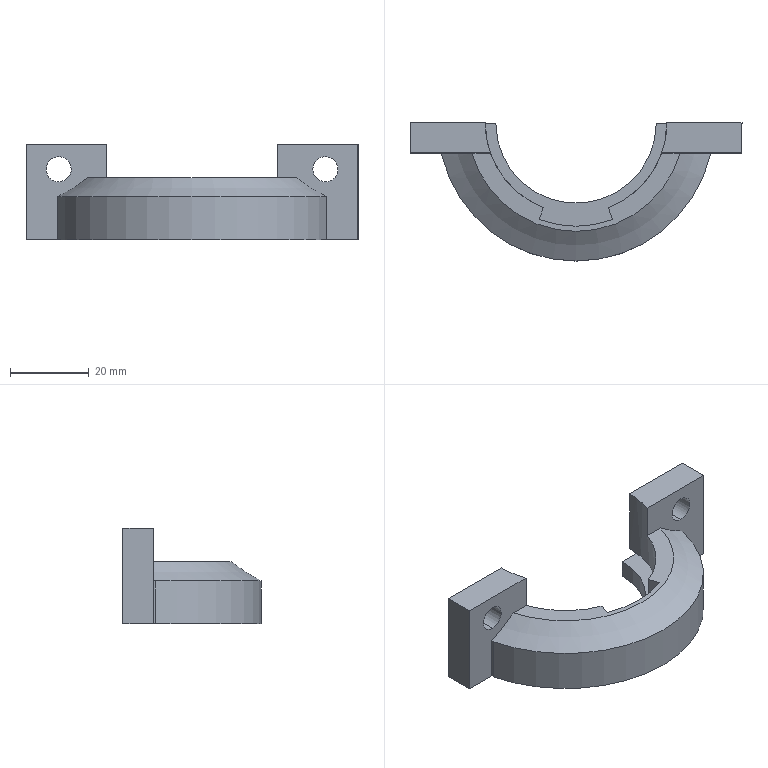Part | SolidWorks | features ICE 14, 3DProfileFeature 1, Cut 1, Extrusion 1, Fillet 1, HoleWzd 1, MirrorPattern 1, MirrorSolid 1, RefAxis 1, RevCut 1, Revolution 1, SewRefSurface 1, Sweep 1, Thicken 1 | 1 solid | 29 faces | box 84.091 x 34.963 x 24.206 mm | volume 18007 mm3 | plane 18 | cylinder 6 | spline 4 | torus 1 | commonest cylinder face diameters 45.974 x2 40.64 x1 52.324 x1 59.436 x1 69.927 x1
STEP:
#1=CARTESIAN_POINT('',(33.782,0.,13.792));
#2=VERTEX_POINT('',#1);
#3=CARTESIAN_POINT('',(33.782,0.,7.442));
#4=VERTEX_POINT('',#3);
#5=CARTESIAN_POINT('',(33.782,0.,13.792));
#6=CARTESIAN_POINT('',(40.132,0.,13.792));
#7=CARTESIAN_POINT('',(40.132,0.,7.442));
#8=CARTESIAN_POINT('',(33.782,0.,7.442));
#9=(BOUNDED_CURVE()B_SPLINE_CURVE(3,(#5,#6,#7,#8),.UNSPECIFIED.,.F.,.F.)B_SPLINE_CURVE_WITH_KNOTS((4,4),(0.,3.142),.UNSPECIFIED.)CURVE()GEOMETRIC_REPRESENTATION_ITEM()RATIONAL_B_SPLINE_CURVE((1.,0.3333,0.3333,1.))REPRESENTATION_ITEM(''));
#10=EDGE_CURVE('',#2,#4,#9,.T.);
#11=ORIENTED_EDGE('',*,*,#10,.T.);
#12=CARTESIAN_POINT('',(33.782,-7.62,7.442));
#13=VERTEX_POINT('',#12);
#14=CARTESIAN_POINT('',(33.782,10.16,7.442));
#15=DIRECTION('',(0.,-1.,0.));
#16=VECTOR('',#15,1000.);
#17=LINE('',#14,#16);
#18=EDGE_CURVE('',#4,#13,#17,.T.);
#19=ORIENTED_EDGE('',*,*,#18,.T.);
#20=CARTESIAN_POINT('',(33.782,-7.62,13.792));
#21=VERTEX_POINT('',#20);
#22=CARTESIAN_POINT('',(33.782,-7.62,13.792));
#23=CARTESIAN_POINT('',(40.132,-7.62,13.792));
#24=CARTESIAN_POINT('',(40.132,-7.62,7.442));
#25=CARTESIAN_POINT('',(33.782,-7.62,7.442));
#26=(BOUNDED_CURVE()B_SPLINE_CURVE(3,(#22,#23,#24,#25),.UNSPECIFIED.,.F.,.F.)B_SPLINE_CURVE_WITH_KNOTS((4,4),(0.,3.142),.UNSPECIFIED.)CURVE()GEOMETRIC_REPRESENTATION_ITEM()RATIONAL_B_SPLINE_CURVE((1.,0.3333,0.3333,1.))REPRESENTATION_ITEM(''));
#27=EDGE_CURVE('',#21,#13,#26,.T.);
#28=ORIENTED_EDGE('',*,*,#27,.F.);
#29=CARTESIAN_POINT('',(33.782,10.16,13.792));
#30=DIRECTION('',(0.,-1.,0.));
#31=VECTOR('',#30,1000.);
#32=LINE('',#29,#31);
#33=EDGE_CURVE('',#2,#21,#32,.T.);
#34=ORIENTED_EDGE('',*,*,#33,.F.);
#35=EDGE_LOOP('',(#11,#19,#28,#34));
#36=FACE_OUTER_BOUND('',#35,.T.);
#37=CARTESIAN_POINT('',(33.782,0.,13.792));
#38=CARTESIAN_POINT('',(33.782,-7.62,13.792));
#39=CARTESIAN_POINT('',(40.132,0.,13.792));
#40=CARTESIAN_POINT('',(40.132,-7.62,13.792));
#41=CARTESIAN_POINT('',(40.132,0.,7.442));
#42=CARTESIAN_POINT('',(40.132,-7.62,7.442));
#43=CARTESIAN_POINT('',(33.782,0.,7.442));
#44=CARTESIAN_POINT('',(33.782,-7.62,7.442));
#45=(BOUNDED_SURFACE()B_SPLINE_SURFACE(3,1,((#37,#38),(#39,#40),(#41,#42),(#43,#44)),.UNSPECIFIED.,.F.,.F.,.T.)B_SPLINE_SURFACE_WITH_KNOTS((4,4),(2,2),(0.,1.),(0.,1.),.UNSPECIFIED.)GEOMETRIC_REPRESENTATION_ITEM()RATIONAL_B_SPLINE_SURFACE(((1.,1.),(0.3333,0.3333),(0.3333,0.3333),(1.,1.)))REPRESENTATION_ITEM('')SURFACE());
#46=ADVANCED_FACE('',(#36),#45,.T.);
#47=CARTESIAN_POINT('',(-33.782,0.,7.442));
#48=VERTEX_POINT('',#47);
#49=CARTESIAN_POINT('',(-33.782,0.,13.792));
#50=VERTEX_POINT('',#49);
#51=CARTESIAN_POINT('',(-33.782,0.,7.442));
#52=CARTESIAN_POINT('',(-27.432,0.,7.442));
#53=CARTESIAN_POINT('',(-27.432,0.,13.792));
#54=CARTESIAN_POINT('',(-33.782,0.,13.792));
#55=(BOUNDED_CURVE()B_SPLINE_CURVE(3,(#51,#52,#53,#54),.UNSPECIFIED.,.F.,.T.)B_SPLINE_CURVE_WITH_KNOTS((4,4),(3.142,6.283),.UNSPECIFIED.)CURVE()GEOMETRIC_REPRESENTATION_ITEM()RATIONAL_B_SPLINE_CURVE((1.,0.3333,0.3333,1.))REPRESENTATION_ITEM(''));
#56=EDGE_CURVE('',#48,#50,#55,.T.);
#57=ORIENTED_EDGE('',*,*,#56,.F.);
#58=CARTESIAN_POINT('',(-33.782,-7.62,7.442));
#59=VERTEX_POINT('',#58);
#60=CARTESIAN_POINT('',(-33.782,10.16,7.442));
#61=DIRECTION('',(0.,-1.,0.));
#62=VECTOR('',#61,1000.);
#63=LINE('',#60,#62);
#64=EDGE_CURVE('',#48,#59,#63,.T.);
#65=ORIENTED_EDGE('',*,*,#64,.T.);
#66=CARTESIAN_POINT('',(-33.782,-7.62,13.792));
#67=VERTEX_POINT('',#66);
#68=CARTESIAN_POINT('',(-33.782,-7.62,7.442));
#69=CARTESIAN_POINT('',(-27.432,-7.62,7.442));
#70=CARTESIAN_POINT('',(-27.432,-7.62,13.792));
#71=CARTESIAN_POINT('',(-33.782,-7.62,13.792));
#72=(BOUNDED_CURVE()B_SPLINE_CURVE(3,(#68,#69,#70,#71),.UNSPECIFIED.,.F.,.T.)B_SPLINE_CURVE_WITH_KNOTS((4,4),(3.142,6.283),.UNSPECIFIED.)CURVE()GEOMETRIC_REPRESENTATION_ITEM()RATIONAL_B_SPLINE_CURVE((1.,0.3333,0.3333,1.))REPRESENTATION_ITEM(''));
#73=EDGE_CURVE('',#59,#67,#72,.T.);
#74=ORIENTED_EDGE('',*,*,#73,.T.);
#75=CARTESIAN_POINT('',(-33.782,10.16,13.792));
#76=DIRECTION('',(0.,-1.,0.));
#77=VECTOR('',#76,1000.);
#78=LINE('',#75,#77);
#79=EDGE_CURVE('',#50,#67,#78,.T.);
#80=ORIENTED_EDGE('',*,*,#79,.F.);
#81=EDGE_LOOP('',(#57,#65,#74,#80));
#82=FACE_OUTER_BOUND('',#81,.T.);
#83=CARTESIAN_POINT('',(-33.782,0.,7.442));
#84=CARTESIAN_POINT('',(-33.782,-7.62,7.442));
#85=CARTESIAN_POINT('',(-27.432,0.,7.442));
#86=CARTESIAN_POINT('',(-27.432,-7.62,7.442));
#87=CARTESIAN_POINT('',(-27.432,0.,13.792));
#88=CARTESIAN_POINT('',(-27.432,-7.62,13.792));
#89=CARTESIAN_POINT('',(-33.782,0.,13.792));
#90=CARTESIAN_POINT('',(-33.782,-7.62,13.792));
#91=(BOUNDED_SURFACE()B_SPLINE_SURFACE(3,1,((#83,#84),(#85,#86),(#87,#88),(#89,#90)),.UNSPECIFIED.,.F.,.F.,.F.)B_SPLINE_SURFACE_WITH_KNOTS((4,4),(2,2),(0.,1.),(0.,1.),.UNSPECIFIED.)GEOMETRIC_REPRESENTATION_ITEM()RATIONAL_B_SPLINE_SURFACE(((1.,1.),(0.3333,0.3333),(0.3333,0.3333),(1.,1.)))REPRESENTATION_ITEM('')SURFACE());
#92=ADVANCED_FACE('',(#82),#91,.F.);
#93=CARTESIAN_POINT('',(20.32,0.,-2.778));
#94=VERTEX_POINT('',#93);
#95=CARTESIAN_POINT('',(-20.32,0.,-2.778));
#96=VERTEX_POINT('',#95);
#97=CARTESIAN_POINT('',(0.,0.,-2.778));
#98=DIRECTION('',(0.,0.,-1.));
#99=DIRECTION('',(1.,0.,0.));
#100=AXIS2_PLACEMENT_3D('',#97,#98,#99);
#101=CIRCLE('',#100,20.32);
#102=EDGE_CURVE('',#94,#96,#101,.T.);
#103=ORIENTED_EDGE('',*,*,#102,.F.);
#104=CARTESIAN_POINT('',(20.32,0.,-7.239));
#105=VERTEX_POINT('',#104);
#106=CARTESIAN_POINT('',(20.32,0.,87.108));
#107=DIRECTION('',(0.,0.,-1.));
#108=VECTOR('',#107,1000.);
#109=LINE('',#106,#108);
#110=EDGE_CURVE('',#94,#105,#109,.T.);
#111=ORIENTED_EDGE('',*,*,#110,.T.);
#112=CARTESIAN_POINT('',(-20.32,0.,-7.239));
#113=VERTEX_POINT('',#112);
#114=CARTESIAN_POINT('',(0.,0.,-7.239));
#115=DIRECTION('',(0.,0.,-1.));
#116=DIRECTION('',(-1.,0.,0.));
#117=AXIS2_PLACEMENT_3D('',#114,#115,#116);
#118=CIRCLE('',#117,20.32);
#119=EDGE_CURVE('',#105,#113,#118,.T.);
#120=ORIENTED_EDGE('',*,*,#119,.T.);
#121=CARTESIAN_POINT('',(-20.32,0.,87.108));
#122=DIRECTION('',(0.,0.,1.));
#123=VECTOR('',#122,1000.);
#124=LINE('',#121,#123);
#125=EDGE_CURVE('',#113,#96,#124,.T.);
#126=ORIENTED_EDGE('',*,*,#125,.T.);
#127=EDGE_LOOP('',(#103,#111,#120,#126));
#128=FACE_OUTER_BOUND('',#127,.T.);
#129=CARTESIAN_POINT('',(0.,0.,87.108));
#130=DIRECTION('',(0.,0.,-1.));
#131=DIRECTION('',(-1.,0.,0.));
#132=AXIS2_PLACEMENT_3D('',#129,#130,#131);
#133=CYLINDRICAL_SURFACE('',#132,20.32);
#134=ADVANCED_FACE('',(#128),#133,.F.);
#135=ORIENTED_EDGE('',*,*,#27,.T.);
#136=CARTESIAN_POINT('',(33.782,-7.62,7.442));
#137=CARTESIAN_POINT('',(27.432,-7.62,7.442));
#138=CARTESIAN_POINT('',(27.432,-7.62,13.792));
#139=CARTESIAN_POINT('',(33.782,-7.62,13.792));
#140=(BOUNDED_CURVE()B_SPLINE_CURVE(3,(#136,#137,#138,#139),.UNSPECIFIED.,.F.,.F.)B_SPLINE_CURVE_WITH_KNOTS((4,4),(3.142,6.283),.UNSPECIFIED.)CURVE()GEOMETRIC_REPRESENTATION_ITEM()RATIONAL_B_SPLINE_CURVE((1.,0.3333,0.3333,1.))REPRESENTATION_ITEM(''));
#141=EDGE_CURVE('',#13,#21,#140,.T.);
#142=ORIENTED_EDGE('',*,*,#141,.T.);
#143=EDGE_LOOP('',(#135,#142));
#144=FACE_BOUND('',#143,.T.);
#145=CARTESIAN_POINT('',(21.687,-7.62,8.484));
#146=VERTEX_POINT('',#145);
#147=CARTESIAN_POINT('',(26.377,-7.62,8.484));
#148=VERTEX_POINT('',#147);
#149=CARTESIAN_POINT('',(0.,-7.62,8.484));
#150=DIRECTION('',(1.,0.,0.));
#151=VECTOR('',#150,1000.);
#152=LINE('',#149,#151);
#153=EDGE_CURVE('',#146,#148,#152,.T.);
#154=ORIENTED_EDGE('',*,*,#153,.T.);
#155=CARTESIAN_POINT('',(33.984,-7.62,3.706));
#156=VERTEX_POINT('',#155);
#157=CARTESIAN_POINT('',(26.377,-7.62,8.484));
#158=CARTESIAN_POINT('',(28.729,-7.62,6.598));
#159=CARTESIAN_POINT('',(31.263,-7.62,5.003));
#160=CARTESIAN_POINT('',(33.984,-7.62,3.706));
#161=B_SPLINE_CURVE_WITH_KNOTS('',3,(#157,#158,#159,#160),.UNSPECIFIED.,.F.,.F.,(4,4),(0.,0.008983),.UNSPECIFIED.);
#162=EDGE_CURVE('',#148,#156,#161,.T.);
#163=ORIENTED_EDGE('',*,*,#162,.T.);
#164=CARTESIAN_POINT('',(33.984,-7.62,-7.239));
#165=VERTEX_POINT('',#164);
#166=CARTESIAN_POINT('',(33.984,-7.62,2.54));
#167=DIRECTION('',(0.,0.,-1.));
#168=VECTOR('',#167,1000.);
#169=LINE('',#166,#168);
#170=EDGE_CURVE('',#156,#165,#169,.T.);
#171=ORIENTED_EDGE('',*,*,#170,.T.);
#172=CARTESIAN_POINT('',(42.02,-7.62,-7.239));
#173=VERTEX_POINT('',#172);
#174=CARTESIAN_POINT('',(0.,-7.62,-7.239));
#175=DIRECTION('',(-1.,0.,0.));
#176=VECTOR('',#175,1000.);
#177=LINE('',#174,#176);
#178=EDGE_CURVE('',#173,#165,#177,.T.);
#179=ORIENTED_EDGE('',*,*,#178,.F.);
#180=CARTESIAN_POINT('',(42.02,-7.62,16.967));
#181=VERTEX_POINT('',#180);
#182=CARTESIAN_POINT('',(42.02,-7.62,16.967));
#183=DIRECTION('',(0.,0.,-1.));
#184=VECTOR('',#183,1000.);
#185=LINE('',#182,#184);
#186=EDGE_CURVE('',#181,#173,#185,.T.);
#187=ORIENTED_EDGE('',*,*,#186,.F.);
#188=CARTESIAN_POINT('',(21.687,-7.62,16.967));
#189=VERTEX_POINT('',#188);
#190=CARTESIAN_POINT('',(0.,-7.62,16.967));
#191=DIRECTION('',(-1.,0.,0.));
#192=VECTOR('',#191,1000.);
#193=LINE('',#190,#192);
#194=EDGE_CURVE('',#181,#189,#193,.T.);
#195=ORIENTED_EDGE('',*,*,#194,.T.);
#196=CARTESIAN_POINT('',(21.687,-7.62,8.484));
#197=DIRECTION('',(0.,0.,1.));
#198=VECTOR('',#197,1000.);
#199=LINE('',#196,#198);
#200=EDGE_CURVE('',#146,#189,#199,.T.);
#201=ORIENTED_EDGE('',*,*,#200,.F.);
#202=EDGE_LOOP('',(#154,#163,#171,#179,#187,#195,#201));
#203=FACE_OUTER_BOUND('',#202,.T.);
#204=CARTESIAN_POINT('',(0.,-7.62,0.));
#205=DIRECTION('',(0.,-1.,0.));
#206=DIRECTION('',(0.,0.,-1.));
#207=AXIS2_PLACEMENT_3D('',#204,#205,#206);
#208=PLANE('',#207);
#209=ADVANCED_FACE('',(#144,#203),#208,.T.);
#210=CARTESIAN_POINT('',(9.312,-24.448,8.484));
#211=VERTEX_POINT('',#210);
#212=CARTESIAN_POINT('',(9.312,-24.448,0.));
#213=VERTEX_POINT('',#212);
#214=CARTESIAN_POINT('',(9.312,-24.448,7.137));
#215=DIRECTION('',(0.,0.,-1.));
#216=VECTOR('',#215,1000.);
#217=LINE('',#214,#216);
#218=EDGE_CURVE('',#211,#213,#217,.T.);
#219=ORIENTED_EDGE('',*,*,#218,.F.);
#220=CARTESIAN_POINT('',(8.182,-21.481,8.484));
#221=VERTEX_POINT('',#220);
#222=CARTESIAN_POINT('',(0.,0.,8.484));
#223=DIRECTION('',(0.356,-0.9345,0.));
#224=VECTOR('',#223,1000.);
#225=LINE('',#222,#224);
#226=EDGE_CURVE('',#221,#211,#225,.T.);
#227=ORIENTED_EDGE('',*,*,#226,.F.);
#228=CARTESIAN_POINT('',(8.182,-21.481,0.));
#229=VERTEX_POINT('',#228);
#230=CARTESIAN_POINT('',(8.182,-21.481,16.967));
#231=DIRECTION('',(0.,0.,1.));
#232=VECTOR('',#231,1000.);
#233=LINE('',#230,#232);
#234=EDGE_CURVE('',#229,#221,#233,.T.);
#235=ORIENTED_EDGE('',*,*,#234,.F.);
#236=CARTESIAN_POINT('',(0.,0.,0.));
#237=DIRECTION('',(0.356,-0.9345,0.));
#238=VECTOR('',#237,1000.);
#239=LINE('',#236,#238);
#240=EDGE_CURVE('',#229,#213,#239,.T.);
#241=ORIENTED_EDGE('',*,*,#240,.T.);
#242=EDGE_LOOP('',(#219,#227,#235,#241));
#243=FACE_OUTER_BOUND('',#242,.T.);
#244=CARTESIAN_POINT('',(0.,0.,-0.8128));
#245=DIRECTION('',(-0.9345,-0.356,0.));
#246=DIRECTION('',(0.356,-0.9345,0.));
#247=AXIS2_PLACEMENT_3D('',#244,#245,#246);
#248=PLANE('',#247);
#249=ADVANCED_FACE('',(#243),#248,.T.);
#250=CARTESIAN_POINT('',(22.987,0.,16.967));
#251=VERTEX_POINT('',#250);
#252=CARTESIAN_POINT('',(0.,0.,16.967));
#253=DIRECTION('',(0.,0.,1.));
#254=DIRECTION('',(1.,0.,0.));
#255=AXIS2_PLACEMENT_3D('',#252,#253,#254);
#256=CIRCLE('',#255,22.987);
#257=EDGE_CURVE('',#189,#251,#256,.T.);
#258=ORIENTED_EDGE('',*,*,#257,.F.);
#259=ORIENTED_EDGE('',*,*,#194,.F.);
#260=CARTESIAN_POINT('',(42.037,0.,16.967));
#261=VERTEX_POINT('',#260);
#262=CARTESIAN_POINT('',(42.037,0.05675,16.967));
#263=DIRECTION('',(-0.002237,-1.,0.));
#264=VECTOR('',#263,1000.);
#265=LINE('',#262,#264);
#266=EDGE_CURVE('',#261,#181,#265,.T.);
#267=ORIENTED_EDGE('',*,*,#266,.F.);
#268=CARTESIAN_POINT('',(0.,0.,16.967));
#269=DIRECTION('',(1.,0.,0.));
#270=VECTOR('',#269,1000.);
#271=LINE('',#268,#270);
#272=EDGE_CURVE('',#251,#261,#271,.T.);
#273=ORIENTED_EDGE('',*,*,#272,.F.);
#274=EDGE_LOOP('',(#258,#259,#267,#273));
#275=FACE_OUTER_BOUND('',#274,.T.);
#276=CARTESIAN_POINT('',(0.,0.,16.967));
#277=DIRECTION('',(0.,0.,1.));
#278=DIRECTION('',(1.,0.,0.));
#279=AXIS2_PLACEMENT_3D('',#276,#277,#278);
#280=PLANE('',#279);
#281=ADVANCED_FACE('',(#275),#280,.T.);
#282=CARTESIAN_POINT('',(0.,0.,8.484));
#283=DIRECTION('',(0.,0.,-1.));
#284=DIRECTION('',(1.,0.,0.));
#285=AXIS2_PLACEMENT_3D('',#282,#283,#284);
#286=CIRCLE('',#285,22.987);
#287=EDGE_CURVE('',#146,#221,#286,.T.);
#288=ORIENTED_EDGE('',*,*,#287,.F.);
#289=ORIENTED_EDGE('',*,*,#200,.T.);
#290=ORIENTED_EDGE('',*,*,#257,.T.);
#291=CARTESIAN_POINT('',(22.987,0.,0.));
#292=VERTEX_POINT('',#291);
#293=CARTESIAN_POINT('',(22.987,0.,16.967));
#294=DIRECTION('',(0.,0.,1.));
#295=VECTOR('',#294,1000.);
#296=LINE('',#293,#295);
#297=EDGE_CURVE('',#292,#251,#296,.T.);
#298=ORIENTED_EDGE('',*,*,#297,.F.);
#299=CARTESIAN_POINT('',(0.,0.,0.));
#300=DIRECTION('',(0.,0.,1.));
#301=DIRECTION('',(1.,0.,0.));
#302=AXIS2_PLACEMENT_3D('',#299,#300,#301);
#303=CIRCLE('',#302,22.987);
#304=EDGE_CURVE('',#229,#292,#303,.T.);
#305=ORIENTED_EDGE('',*,*,#304,.F.);
#306=ORIENTED_EDGE('',*,*,#234,.T.);
#307=EDGE_LOOP('',(#288,#289,#290,#298,#305,#306));
#308=FACE_OUTER_BOUND('',#307,.T.);
#309=CARTESIAN_POINT('',(0.,0.,16.967));
#310=DIRECTION('',(0.,0.,-1.));
#311=DIRECTION('',(-1.,0.,0.));
#312=AXIS2_PLACEMENT_3D('',#309,#310,#311);
#313=CYLINDRICAL_SURFACE('',#312,22.987);
#314=ADVANCED_FACE('',(#308),#313,.F.);
#315=CARTESIAN_POINT('',(-9.312,-24.448,8.484));
#316=VERTEX_POINT('',#315);
#317=CARTESIAN_POINT('',(-8.293,-21.439,8.484));
#318=VERTEX_POINT('',#317);
#319=CARTESIAN_POINT('',(-0.921,0.3121,8.484));
#320=DIRECTION('',(0.321,0.9471,0.));
#321=VECTOR('',#320,1000.);
#322=LINE('',#319,#321);
#323=EDGE_CURVE('',#316,#318,#322,.T.);
#324=ORIENTED_EDGE('',*,*,#323,.F.);
#325=CARTESIAN_POINT('',(-9.312,-24.448,0.));
#326=VERTEX_POINT('',#325);
#327=CARTESIAN_POINT('',(-9.312,-24.448,7.137));
#328=DIRECTION('',(0.,0.,-1.));
#329=VECTOR('',#328,1000.);
#330=LINE('',#327,#329);
#331=EDGE_CURVE('',#316,#326,#330,.T.);
#332=ORIENTED_EDGE('',*,*,#331,.T.);
#333=CARTESIAN_POINT('',(-8.293,-21.439,0.));
#334=VERTEX_POINT('',#333);
#335=CARTESIAN_POINT('',(-0.921,0.3121,0.));
#336=DIRECTION('',(-0.321,-0.9471,0.));
#337=VECTOR('',#336,1000.);
#338=LINE('',#335,#337);
#339=EDGE_CURVE('',#334,#326,#338,.T.);
#340=ORIENTED_EDGE('',*,*,#339,.F.);
#341=CARTESIAN_POINT('',(-8.293,-21.439,16.967));
#342=DIRECTION('',(0.,0.,1.));
#343=VECTOR('',#342,1000.);
#344=LINE('',#341,#343);
#345=EDGE_CURVE('',#334,#318,#344,.T.);
#346=ORIENTED_EDGE('',*,*,#345,.T.);
#347=EDGE_LOOP('',(#324,#332,#340,#346));
#348=FACE_OUTER_BOUND('',#347,.T.);
#349=CARTESIAN_POINT('',(-0.921,0.3121,-0.8128));
#350=DIRECTION('',(-0.9471,0.321,0.));
#351=DIRECTION('',(-0.321,-0.9471,0.));
#352=AXIS2_PLACEMENT_3D('',#349,#350,#351);
#353=PLANE('',#352);
#354=ADVANCED_FACE('',(#348),#353,.F.);
#355=CARTESIAN_POINT('',(-42.054,-7.62,16.967));
#356=VERTEX_POINT('',#355);
#357=CARTESIAN_POINT('',(-21.687,-7.62,16.967));
#358=VERTEX_POINT('',#357);
#359=CARTESIAN_POINT('',(0.,-7.62,16.967));
#360=DIRECTION('',(1.,0.,0.));
#361=VECTOR('',#360,1000.);
#362=LINE('',#359,#361);
#363=EDGE_CURVE('',#356,#358,#362,.T.);
#364=ORIENTED_EDGE('',*,*,#363,.T.);
#365=CARTESIAN_POINT('',(-22.987,0.,16.967));
#366=VERTEX_POINT('',#365);
#367=CARTESIAN_POINT('',(0.,0.,16.967));
#368=DIRECTION('',(0.,0.,1.));
#369=DIRECTION('',(1.,0.,0.));
#370=AXIS2_PLACEMENT_3D('',#367,#368,#369);
#371=CIRCLE('',#370,22.987);
#372=EDGE_CURVE('',#366,#358,#371,.T.);
#373=ORIENTED_EDGE('',*,*,#372,.F.);
#374=CARTESIAN_POINT('',(-42.037,0.,16.967));
#375=VERTEX_POINT('',#374);
#376=CARTESIAN_POINT('',(0.,0.,16.967));
#377=DIRECTION('',(1.,0.,0.));
#378=VECTOR('',#377,1000.);
#379=LINE('',#376,#378);
#380=EDGE_CURVE('',#375,#366,#379,.T.);
#381=ORIENTED_EDGE('',*,*,#380,.F.);
#382=CARTESIAN_POINT('',(-42.054,-7.677,16.967));
#383=DIRECTION('',(-0.002237,-1.,0.));
#384=VECTOR('',#383,1000.);
#385=LINE('',#382,#384);
#386=EDGE_CURVE('',#375,#356,#385,.T.);
#387=ORIENTED_EDGE('',*,*,#386,.T.);
#388=EDGE_LOOP('',(#364,#373,#381,#387));
#389=FACE_OUTER_BOUND('',#388,.T.);
#390=CARTESIAN_POINT('',(0.,0.,16.967));
#391=DIRECTION('',(0.,0.,1.));
#392=DIRECTION('',(1.,0.,0.));
#393=AXIS2_PLACEMENT_3D('',#390,#391,#392);
#394=PLANE('',#393);
#395=ADVANCED_FACE('',(#389),#394,.T.);
#396=ORIENTED_EDGE('',*,*,#372,.T.);
#397=CARTESIAN_POINT('',(-21.687,-7.62,8.484));
#398=VERTEX_POINT('',#397);
#399=CARTESIAN_POINT('',(-21.687,-7.62,8.484));
#400=DIRECTION('',(0.,0.,1.));
#401=VECTOR('',#400,1000.);
#402=LINE('',#399,#401);
#403=EDGE_CURVE('',#398,#358,#402,.T.);
#404=ORIENTED_EDGE('',*,*,#403,.F.);
#405=CARTESIAN_POINT('',(0.,0.,8.484));
#406=DIRECTION('',(0.,0.,1.));
#407=DIRECTION('',(1.,0.,0.));
#408=AXIS2_PLACEMENT_3D('',#405,#406,#407);
#409=CIRCLE('',#408,22.987);
#410=EDGE_CURVE('',#398,#318,#409,.T.);
#411=ORIENTED_EDGE('',*,*,#410,.T.);
#412=ORIENTED_EDGE('',*,*,#345,.F.);
#413=CARTESIAN_POINT('',(-22.987,0.,0.));
#414=VERTEX_POINT('',#413);
#415=CARTESIAN_POINT('',(0.,0.,0.));
#416=DIRECTION('',(0.,0.,1.));
#417=DIRECTION('',(1.,0.,0.));
#418=AXIS2_PLACEMENT_3D('',#415,#416,#417);
#419=CIRCLE('',#418,22.987);
#420=EDGE_CURVE('',#414,#334,#419,.T.);
#421=ORIENTED_EDGE('',*,*,#420,.F.);
#422=CARTESIAN_POINT('',(-22.987,0.,16.967));
#423=DIRECTION('',(0.,0.,-1.));
#424=VECTOR('',#423,1000.);
#425=LINE('',#422,#424);
#426=EDGE_CURVE('',#366,#414,#425,.T.);
#427=ORIENTED_EDGE('',*,*,#426,.F.);
#428=EDGE_LOOP('',(#396,#404,#411,#412,#421,#427));
#429=FACE_OUTER_BOUND('',#428,.T.);
#430=CARTESIAN_POINT('',(0.,0.,16.967));
#431=DIRECTION('',(0.,0.,-1.));
#432=DIRECTION('',(-1.,0.,0.));
#433=AXIS2_PLACEMENT_3D('',#430,#431,#432);
#434=CYLINDRICAL_SURFACE('',#433,22.987);
#435=ADVANCED_FACE('',(#429),#434,.F.);
#436=CARTESIAN_POINT('',(-33.782,-7.62,13.792));
#437=CARTESIAN_POINT('',(-40.132,-7.62,13.792));
#438=CARTESIAN_POINT('',(-40.132,-7.62,7.442));
#439=CARTESIAN_POINT('',(-33.782,-7.62,7.442));
#440=(BOUNDED_CURVE()B_SPLINE_CURVE(3,(#436,#437,#438,#439),.UNSPECIFIED.,.F.,.T.)B_SPLINE_CURVE_WITH_KNOTS((4,4),(0.,3.142),.UNSPECIFIED.)CURVE()GEOMETRIC_REPRESENTATION_ITEM()RATIONAL_B_SPLINE_CURVE((1.,0.3333,0.3333,1.))REPRESENTATION_ITEM(''));
#441=EDGE_CURVE('',#67,#59,#440,.T.);
#442=ORIENTED_EDGE('',*,*,#441,.F.);
#443=ORIENTED_EDGE('',*,*,#73,.F.);
#444=EDGE_LOOP('',(#442,#443));
#445=FACE_BOUND('',#444,.T.);
#446=CARTESIAN_POINT('',(-33.984,-7.62,3.706));
#447=VERTEX_POINT('',#446);
#448=CARTESIAN_POINT('',(-33.984,-7.62,-7.239));
#449=VERTEX_POINT('',#448);
#450=CARTESIAN_POINT('',(-33.984,-7.62,2.54));
#451=DIRECTION('',(0.,0.,-1.));
#452=VECTOR('',#451,1000.);
#453=LINE('',#450,#452);
#454=EDGE_CURVE('',#447,#449,#453,.T.);
#455=ORIENTED_EDGE('',*,*,#454,.F.);
#456=CARTESIAN_POINT('',(-26.377,-7.62,8.484));
#457=VERTEX_POINT('',#456);
#458=CARTESIAN_POINT('',(-33.984,-7.62,3.706));
#459=CARTESIAN_POINT('',(-31.263,-7.62,5.003));
#460=CARTESIAN_POINT('',(-28.729,-7.62,6.598));
#461=CARTESIAN_POINT('',(-26.377,-7.62,8.484));
#462=B_SPLINE_CURVE_WITH_KNOTS('',3,(#458,#459,#460,#461),.UNSPECIFIED.,.F.,.F.,(4,4),(0.,0.008983),.UNSPECIFIED.);
#463=EDGE_CURVE('',#447,#457,#462,.T.);
#464=ORIENTED_EDGE('',*,*,#463,.T.);
#465=CARTESIAN_POINT('',(0.,-7.62,8.484));
#466=DIRECTION('',(1.,0.,0.));
#467=VECTOR('',#466,1000.);
#468=LINE('',#465,#467);
#469=EDGE_CURVE('',#457,#398,#468,.T.);
#470=ORIENTED_EDGE('',*,*,#469,.T.);
#471=ORIENTED_EDGE('',*,*,#403,.T.);
#472=ORIENTED_EDGE('',*,*,#363,.F.);
#473=CARTESIAN_POINT('',(-42.054,-7.62,-7.239));
#474=VERTEX_POINT('',#473);
#475=CARTESIAN_POINT('',(-42.054,-7.62,-7.239));
#476=DIRECTION('',(0.,0.,-1.));
#477=VECTOR('',#476,1000.);
#478=LINE('',#475,#477);
#479=EDGE_CURVE('',#356,#474,#478,.T.);
#480=ORIENTED_EDGE('',*,*,#479,.T.);
#481=CARTESIAN_POINT('',(0.,-7.62,-7.239));
#482=DIRECTION('',(1.,0.,0.));
#483=VECTOR('',#482,1000.);
#484=LINE('',#481,#483);
#485=EDGE_CURVE('',#474,#449,#484,.T.);
#486=ORIENTED_EDGE('',*,*,#485,.T.);
#487=EDGE_LOOP('',(#455,#464,#470,#471,#472,#480,#486));
#488=FACE_OUTER_BOUND('',#487,.T.);
#489=CARTESIAN_POINT('',(0.,-7.62,0.));
#490=DIRECTION('',(0.,-1.,0.));
#491=DIRECTION('',(0.,0.,-1.));
#492=AXIS2_PLACEMENT_3D('',#489,#490,#491);
#493=PLANE('',#492);
#494=ADVANCED_FACE('',(#445,#488),#493,.T.);
#495=ORIENTED_EDGE('',*,*,#240,.F.);
#496=ORIENTED_EDGE('',*,*,#304,.T.);
#497=CARTESIAN_POINT('',(29.582,0.,0.));
#498=VERTEX_POINT('',#497);
#499=CARTESIAN_POINT('',(0.,0.,0.));
#500=DIRECTION('',(1.,0.,0.));
#501=VECTOR('',#500,1000.);
#502=LINE('',#499,#501);
#503=EDGE_CURVE('',#292,#498,#502,.T.);
#504=ORIENTED_EDGE('',*,*,#503,.T.);
#505=CARTESIAN_POINT('',(29.582,-2.845,0.));
#506=VERTEX_POINT('',#505);
#507=CARTESIAN_POINT('',(29.582,0.,0.));
#508=DIRECTION('',(0.,1.,0.));
#509=VECTOR('',#508,1000.);
#510=LINE('',#507,#509);
#511=EDGE_CURVE('',#506,#498,#510,.T.);
#512=ORIENTED_EDGE('',*,*,#511,.F.);
#513=CARTESIAN_POINT('',(-29.582,-2.845,0.));
#514=VERTEX_POINT('',#513);
#515=CARTESIAN_POINT('',(0.,0.,0.));
#516=DIRECTION('',(0.,0.,1.));
#517=DIRECTION('',(1.,0.,0.));
#518=AXIS2_PLACEMENT_3D('',#515,#516,#517);
#519=CIRCLE('',#518,29.718);
#520=EDGE_CURVE('',#514,#506,#519,.T.);
#521=ORIENTED_EDGE('',*,*,#520,.F.);
#522=CARTESIAN_POINT('',(-29.582,0.,0.));
#523=VERTEX_POINT('',#522);
#524=CARTESIAN_POINT('',(-29.582,0.,0.));
#525=DIRECTION('',(0.,1.,0.));
#526=VECTOR('',#525,1000.);
#527=LINE('',#524,#526);
#528=EDGE_CURVE('',#514,#523,#527,.T.);
#529=ORIENTED_EDGE('',*,*,#528,.T.);
#530=CARTESIAN_POINT('',(0.,0.,0.));
#531=DIRECTION('',(1.,0.,0.));
#532=VECTOR('',#531,1000.);
#533=LINE('',#530,#532);
#534=EDGE_CURVE('',#523,#414,#533,.T.);
#535=ORIENTED_EDGE('',*,*,#534,.T.);
#536=ORIENTED_EDGE('',*,*,#420,.T.);
#537=ORIENTED_EDGE('',*,*,#339,.T.);
#538=CARTESIAN_POINT('',(0.,0.,0.));
#539=DIRECTION('',(0.,0.,-1.));
#540=DIRECTION('',(-1.,0.,0.));
#541=AXIS2_PLACEMENT_3D('',#538,#539,#540);
#542=CIRCLE('',#541,26.162);
#543=EDGE_CURVE('',#213,#326,#542,.T.);
#544=ORIENTED_EDGE('',*,*,#543,.F.);
#545=EDGE_LOOP('',(#495,#496,#504,#512,#521,#529,#535,#536,#537,#544));
#546=FACE_OUTER_BOUND('',#545,.T.);
#547=CARTESIAN_POINT('',(0.,0.,0.));
#548=DIRECTION('',(0.,0.,1.));
#549=DIRECTION('',(1.,0.,0.));
#550=AXIS2_PLACEMENT_3D('',#547,#548,#549);
#551=PLANE('',#550);
#552=ADVANCED_FACE('',(#546),#551,.F.);
#553=CARTESIAN_POINT('',(-33.984,-8.217,-7.239));
#554=VERTEX_POINT('',#553);
#555=CARTESIAN_POINT('',(-33.984,0.,-7.239));
#556=DIRECTION('',(0.,1.,0.));
#557=VECTOR('',#556,1000.);
#558=LINE('',#555,#557);
#559=EDGE_CURVE('',#554,#449,#558,.T.);
#560=ORIENTED_EDGE('',*,*,#559,.T.);
#561=ORIENTED_EDGE('',*,*,#485,.F.);
#562=CARTESIAN_POINT('',(-42.037,0.,-7.239));
#563=VERTEX_POINT('',#562);
#564=CARTESIAN_POINT('',(-42.037,-0.05678,-7.239));
#565=DIRECTION('',(0.002237,1.,0.));
#566=VECTOR('',#565,1000.);
#567=LINE('',#564,#566);
#568=EDGE_CURVE('',#474,#563,#567,.T.);
#569=ORIENTED_EDGE('',*,*,#568,.T.);
#570=CARTESIAN_POINT('',(0.,0.,-7.239));
#571=DIRECTION('',(1.,0.,0.));
#572=VECTOR('',#571,1000.);
#573=LINE('',#570,#572);
#574=EDGE_CURVE('',#563,#113,#573,.T.);
#575=ORIENTED_EDGE('',*,*,#574,.T.);
#576=ORIENTED_EDGE('',*,*,#119,.F.);
#577=CARTESIAN_POINT('',(42.037,0.,-7.239));
#578=VERTEX_POINT('',#577);
#579=CARTESIAN_POINT('',(0.,0.,-7.239));
#580=DIRECTION('',(1.,0.,0.));
#581=VECTOR('',#580,1000.);
#582=LINE('',#579,#581);
#583=EDGE_CURVE('',#105,#578,#582,.T.);
#584=ORIENTED_EDGE('',*,*,#583,.T.);
#585=CARTESIAN_POINT('',(42.02,-7.563,-7.239));
#586=DIRECTION('',(0.002237,1.,0.));
#587=VECTOR('',#586,1000.);
#588=LINE('',#585,#587);
#589=EDGE_CURVE('',#173,#578,#588,.T.);
#590=ORIENTED_EDGE('',*,*,#589,.F.);
#591=ORIENTED_EDGE('',*,*,#178,.T.);
#592=CARTESIAN_POINT('',(33.984,-8.217,-7.239));
#593=VERTEX_POINT('',#592);
#594=CARTESIAN_POINT('',(33.984,0.,-7.239));
#595=DIRECTION('',(0.,1.,0.));
#596=VECTOR('',#595,1000.);
#597=LINE('',#594,#596);
#598=EDGE_CURVE('',#593,#165,#597,.T.);
#599=ORIENTED_EDGE('',*,*,#598,.F.);
#600=CARTESIAN_POINT('',(0.,0.,-7.239));
#601=DIRECTION('',(0.,0.,-1.));
#602=DIRECTION('',(1.,0.,0.));
#603=AXIS2_PLACEMENT_3D('',#600,#601,#602);
#604=CIRCLE('',#603,34.963);
#605=EDGE_CURVE('',#593,#554,#604,.T.);
#606=ORIENTED_EDGE('',*,*,#605,.T.);
#607=EDGE_LOOP('',(#560,#561,#569,#575,#576,#584,#590,#591,#599,#606));
#608=FACE_OUTER_BOUND('',#607,.T.);
#609=CARTESIAN_POINT('',(0.,0.,-7.239));
#610=DIRECTION('',(0.,0.,-1.));
#611=DIRECTION('',(-1.,0.,0.));
#612=AXIS2_PLACEMENT_3D('',#609,#610,#611);
#613=PLANE('',#612);
#614=ADVANCED_FACE('',(#608),#613,.T.);
#615=CARTESIAN_POINT('',(29.582,-2.845,-2.778));
#616=VERTEX_POINT('',#615);
#617=CARTESIAN_POINT('',(29.582,-2.845,16.967));
#618=DIRECTION('',(0.,0.,-1.));
#619=VECTOR('',#618,1000.);
#620=LINE('',#617,#619);
#621=EDGE_CURVE('',#506,#616,#620,.T.);
#622=ORIENTED_EDGE('',*,*,#621,.T.);
#623=CARTESIAN_POINT('',(-29.582,-2.845,-2.778));
#624=VERTEX_POINT('',#623);
#625=CARTESIAN_POINT('',(0.,0.,-2.778));
#626=DIRECTION('',(0.,0.,1.));
#627=DIRECTION('',(1.,0.,0.));
#628=AXIS2_PLACEMENT_3D('',#625,#626,#627);
#629=CIRCLE('',#628,29.718);
#630=EDGE_CURVE('',#624,#616,#629,.T.);
#631=ORIENTED_EDGE('',*,*,#630,.F.);
#632=CARTESIAN_POINT('',(-29.582,-2.845,16.967));
#633=DIRECTION('',(0.,0.,-1.));
#634=VECTOR('',#633,1000.);
#635=LINE('',#632,#634);
#636=EDGE_CURVE('',#514,#624,#635,.T.);
#637=ORIENTED_EDGE('',*,*,#636,.F.);
#638=ORIENTED_EDGE('',*,*,#520,.T.);
#639=EDGE_LOOP('',(#622,#631,#637,#638));
#640=FACE_OUTER_BOUND('',#639,.T.);
#641=CARTESIAN_POINT('',(0.,0.,16.967));
#642=DIRECTION('',(0.,0.,1.));
#643=DIRECTION('',(1.,0.,0.));
#644=AXIS2_PLACEMENT_3D('',#641,#642,#643);
#645=CYLINDRICAL_SURFACE('',#644,29.718);
#646=ADVANCED_FACE('',(#640),#645,.F.);
#647=CARTESIAN_POINT('',(-33.782,0.,13.792));
#648=CARTESIAN_POINT('',(-40.132,0.,13.792));
#649=CARTESIAN_POINT('',(-40.132,0.,7.442));
#650=CARTESIAN_POINT('',(-33.782,0.,7.442));
#651=(BOUNDED_CURVE()B_SPLINE_CURVE(3,(#647,#648,#649,#650),.UNSPECIFIED.,.F.,.T.)B_SPLINE_CURVE_WITH_KNOTS((4,4),(0.,3.142),.UNSPECIFIED.)CURVE()GEOMETRIC_REPRESENTATION_ITEM()RATIONAL_B_SPLINE_CURVE((1.,0.3333,0.3333,1.))REPRESENTATION_ITEM(''));
#652=EDGE_CURVE('',#50,#48,#651,.T.);
#653=ORIENTED_EDGE('',*,*,#652,.T.);
#654=ORIENTED_EDGE('',*,*,#56,.T.);
#655=EDGE_LOOP('',(#653,#654));
#656=FACE_BOUND('',#655,.T.);
#657=CARTESIAN_POINT('',(-29.582,0.,-2.778));
#658=VERTEX_POINT('',#657);
#659=CARTESIAN_POINT('',(-29.582,0.,0.));
#660=DIRECTION('',(0.,0.,1.));
#661=VECTOR('',#660,1000.);
#662=LINE('',#659,#661);
#663=EDGE_CURVE('',#658,#523,#662,.T.);
#664=ORIENTED_EDGE('',*,*,#663,.F.);
#665=CARTESIAN_POINT('',(-20.32,0.,-2.778));
#666=DIRECTION('',(-1.,0.,0.));
#667=VECTOR('',#666,1000.);
#668=LINE('',#665,#667);
#669=EDGE_CURVE('',#96,#658,#668,.T.);
#670=ORIENTED_EDGE('',*,*,#669,.F.);
#671=ORIENTED_EDGE('',*,*,#125,.F.);
#672=ORIENTED_EDGE('',*,*,#574,.F.);
#673=CARTESIAN_POINT('',(-42.037,0.,16.967));
#674=DIRECTION('',(0.,0.,1.));
#675=VECTOR('',#674,1000.);
#676=LINE('',#673,#675);
#677=EDGE_CURVE('',#563,#375,#676,.T.);
#678=ORIENTED_EDGE('',*,*,#677,.T.);
#679=ORIENTED_EDGE('',*,*,#380,.T.);
#680=ORIENTED_EDGE('',*,*,#426,.T.);
#681=ORIENTED_EDGE('',*,*,#534,.F.);
#682=EDGE_LOOP('',(#664,#670,#671,#672,#678,#679,#680,#681));
#683=FACE_OUTER_BOUND('',#682,.T.);
#684=CARTESIAN_POINT('',(0.,0.,-7.239));
#685=DIRECTION('',(0.,-1.,0.));
#686=DIRECTION('',(0.,0.,-1.));
#687=AXIS2_PLACEMENT_3D('',#684,#685,#686);
#688=PLANE('',#687);
#689=ADVANCED_FACE('',(#656,#683),#688,.F.);
#690=ORIENTED_EDGE('',*,*,#10,.F.);
#691=CARTESIAN_POINT('',(33.782,0.,7.442));
#692=CARTESIAN_POINT('',(27.432,0.,7.442));
#693=CARTESIAN_POINT('',(27.432,0.,13.792));
#694=CARTESIAN_POINT('',(33.782,0.,13.792));
#695=(BOUNDED_CURVE()B_SPLINE_CURVE(3,(#691,#692,#693,#694),.UNSPECIFIED.,.F.,.T.)B_SPLINE_CURVE_WITH_KNOTS((4,4),(3.142,6.283),.UNSPECIFIED.)CURVE()GEOMETRIC_REPRESENTATION_ITEM()RATIONAL_B_SPLINE_CURVE((1.,0.3333,0.3333,1.))REPRESENTATION_ITEM(''));
#696=EDGE_CURVE('',#4,#2,#695,.T.);
#697=ORIENTED_EDGE('',*,*,#696,.F.);
#698=EDGE_LOOP('',(#690,#697));
#699=FACE_BOUND('',#698,.T.);
#700=CARTESIAN_POINT('',(29.582,0.,-2.778));
#701=VERTEX_POINT('',#700);
#702=CARTESIAN_POINT('',(29.582,0.,-2.778));
#703=DIRECTION('',(-1.,0.,0.));
#704=VECTOR('',#703,1000.);
#705=LINE('',#702,#704);
#706=EDGE_CURVE('',#701,#94,#705,.T.);
#707=ORIENTED_EDGE('',*,*,#706,.F.);
#708=CARTESIAN_POINT('',(29.582,0.,0.));
#709=DIRECTION('',(0.,0.,1.));
#710=VECTOR('',#709,1000.);
#711=LINE('',#708,#710);
#712=EDGE_CURVE('',#701,#498,#711,.T.);
#713=ORIENTED_EDGE('',*,*,#712,.T.);
#714=ORIENTED_EDGE('',*,*,#503,.F.);
#715=ORIENTED_EDGE('',*,*,#297,.T.);
#716=ORIENTED_EDGE('',*,*,#272,.T.);
#717=CARTESIAN_POINT('',(42.037,0.,-7.239));
#718=DIRECTION('',(0.,0.,1.));
#719=VECTOR('',#718,1000.);
#720=LINE('',#717,#719);
#721=EDGE_CURVE('',#578,#261,#720,.T.);
#722=ORIENTED_EDGE('',*,*,#721,.F.);
#723=ORIENTED_EDGE('',*,*,#583,.F.);
#724=ORIENTED_EDGE('',*,*,#110,.F.);
#725=EDGE_LOOP('',(#707,#713,#714,#715,#716,#722,#723,#724));
#726=FACE_OUTER_BOUND('',#725,.T.);
#727=CARTESIAN_POINT('',(0.,0.,-7.239));
#728=DIRECTION('',(0.,-1.,0.));
#729=DIRECTION('',(0.,0.,-1.));
#730=AXIS2_PLACEMENT_3D('',#727,#728,#729);
#731=PLANE('',#730);
#732=ADVANCED_FACE('',(#699,#726),#731,.F.);
#733=ORIENTED_EDGE('',*,*,#636,.T.);
#734=CARTESIAN_POINT('',(-29.582,0.,-2.778));
#735=DIRECTION('',(0.,-1.,0.));
#736=VECTOR('',#735,1000.);
#737=LINE('',#734,#736);
#738=EDGE_CURVE('',#658,#624,#737,.T.);
#739=ORIENTED_EDGE('',*,*,#738,.F.);
#740=ORIENTED_EDGE('',*,*,#663,.T.);
#741=ORIENTED_EDGE('',*,*,#528,.F.);
#742=EDGE_LOOP('',(#733,#739,#740,#741));
#743=FACE_OUTER_BOUND('',#742,.T.);
#744=CARTESIAN_POINT('',(-29.582,0.,0.));
#745=DIRECTION('',(1.,0.,0.));
#746=DIRECTION('',(0.,0.,-1.));
#747=AXIS2_PLACEMENT_3D('',#744,#745,#746);
#748=PLANE('',#747);
#749=ADVANCED_FACE('',(#743),#748,.T.);
#750=ORIENTED_EDGE('',*,*,#621,.F.);
#751=ORIENTED_EDGE('',*,*,#511,.T.);
#752=ORIENTED_EDGE('',*,*,#712,.F.);
#753=CARTESIAN_POINT('',(29.582,-2.845,-2.778));
#754=DIRECTION('',(0.,1.,0.));
#755=VECTOR('',#754,1000.);
#756=LINE('',#753,#755);
#757=EDGE_CURVE('',#616,#701,#756,.T.);
#758=ORIENTED_EDGE('',*,*,#757,.F.);
#759=EDGE_LOOP('',(#750,#751,#752,#758));
#760=FACE_OUTER_BOUND('',#759,.T.);
#761=CARTESIAN_POINT('',(29.582,0.,0.));
#762=DIRECTION('',(-1.,0.,0.));
#763=DIRECTION('',(0.,0.,-1.));
#764=AXIS2_PLACEMENT_3D('',#761,#762,#763);
#765=PLANE('',#764);
#766=ADVANCED_FACE('',(#760),#765,.T.);
#767=ORIENTED_EDGE('',*,*,#543,.T.);
#768=ORIENTED_EDGE('',*,*,#331,.F.);
#769=CARTESIAN_POINT('',(0.,0.,8.484));
#770=DIRECTION('',(0.,0.,-1.));
#771=DIRECTION('',(1.,0.,0.));
#772=AXIS2_PLACEMENT_3D('',#769,#770,#771);
#773=CIRCLE('',#772,26.162);
#774=EDGE_CURVE('',#211,#316,#773,.T.);
#775=ORIENTED_EDGE('',*,*,#774,.F.);
#776=ORIENTED_EDGE('',*,*,#218,.T.);
#777=EDGE_LOOP('',(#767,#768,#775,#776));
#778=FACE_OUTER_BOUND('',#777,.T.);
#779=CARTESIAN_POINT('',(0.,0.,7.137));
#780=DIRECTION('',(0.,0.,-1.));
#781=DIRECTION('',(-1.,0.,0.));
#782=AXIS2_PLACEMENT_3D('',#779,#780,#781);
#783=CYLINDRICAL_SURFACE('',#782,26.162);
#784=ADVANCED_FACE('',(#778),#783,.F.);
#785=ORIENTED_EDGE('',*,*,#469,.F.);
#786=CARTESIAN_POINT('',(0.,0.,8.484));
#787=DIRECTION('',(0.,0.,1.));
#788=DIRECTION('',(-1.,0.,0.));
#789=AXIS2_PLACEMENT_3D('',#786,#787,#788);
#790=CIRCLE('',#789,27.456);
#791=EDGE_CURVE('',#457,#148,#790,.T.);
#792=ORIENTED_EDGE('',*,*,#791,.T.);
#793=ORIENTED_EDGE('',*,*,#153,.F.);
#794=ORIENTED_EDGE('',*,*,#287,.T.);
#795=ORIENTED_EDGE('',*,*,#226,.T.);
#796=ORIENTED_EDGE('',*,*,#774,.T.);
#797=ORIENTED_EDGE('',*,*,#323,.T.);
#798=ORIENTED_EDGE('',*,*,#410,.F.);
#799=EDGE_LOOP('',(#785,#792,#793,#794,#795,#796,#797,#798));
#800=FACE_OUTER_BOUND('',#799,.T.);
#801=CARTESIAN_POINT('',(0.,0.,8.484));
#802=DIRECTION('',(0.,0.,1.));
#803=DIRECTION('',(1.,0.,0.));
#804=AXIS2_PLACEMENT_3D('',#801,#802,#803);
#805=PLANE('',#804);
#806=ADVANCED_FACE('',(#800),#805,.T.);
#807=ORIENTED_EDGE('',*,*,#605,.F.);
#808=CARTESIAN_POINT('',(33.984,-8.217,3.64));
#809=VERTEX_POINT('',#808);
#810=CARTESIAN_POINT('',(33.984,-8.217,-74.974));
#811=DIRECTION('',(0.,0.,1.));
#812=VECTOR('',#811,1000.);
#813=LINE('',#810,#812);
#814=EDGE_CURVE('',#593,#809,#813,.T.);
#815=ORIENTED_EDGE('',*,*,#814,.T.);
#816=CARTESIAN_POINT('',(-33.984,-8.217,3.64));
#817=VERTEX_POINT('',#816);
#818=CARTESIAN_POINT('',(0.,0.,3.64));
#819=DIRECTION('',(0.,0.,-1.));
#820=DIRECTION('',(-1.,0.,0.));
#821=AXIS2_PLACEMENT_3D('',#818,#819,#820);
#822=CIRCLE('',#821,34.963);
#823=EDGE_CURVE('',#809,#817,#822,.T.);
#824=ORIENTED_EDGE('',*,*,#823,.T.);
#825=CARTESIAN_POINT('',(-33.984,-8.217,-74.974));
#826=DIRECTION('',(0.,0.,1.));
#827=VECTOR('',#826,1000.);
#828=LINE('',#825,#827);
#829=EDGE_CURVE('',#554,#817,#828,.T.);
#830=ORIENTED_EDGE('',*,*,#829,.F.);
#831=EDGE_LOOP('',(#807,#815,#824,#830));
#832=FACE_OUTER_BOUND('',#831,.T.);
#833=CARTESIAN_POINT('',(0.,0.,-74.974));
#834=DIRECTION('',(0.,0.,1.));
#835=DIRECTION('',(1.,0.,0.));
#836=AXIS2_PLACEMENT_3D('',#833,#834,#835);
#837=CYLINDRICAL_SURFACE('',#836,34.963);
#838=ADVANCED_FACE('',(#832),#837,.T.);
#839=ORIENTED_EDGE('',*,*,#829,.T.);
#840=CARTESIAN_POINT('',(-33.984,-8.217,3.64));
#841=CARTESIAN_POINT('',(-33.984,-8.018,3.663));
#842=CARTESIAN_POINT('',(-33.984,-7.819,3.685));
#843=CARTESIAN_POINT('',(-33.984,-7.62,3.706));
#844=B_SPLINE_CURVE_WITH_KNOTS('',3,(#840,#841,#842,#843),.UNSPECIFIED.,.F.,.F.,(4,4),(0.,0.0006006),.UNSPECIFIED.);
#845=EDGE_CURVE('',#817,#447,#844,.T.);
#846=ORIENTED_EDGE('',*,*,#845,.T.);
#847=ORIENTED_EDGE('',*,*,#454,.T.);
#848=ORIENTED_EDGE('',*,*,#559,.F.);
#849=EDGE_LOOP('',(#839,#846,#847,#848));
#850=FACE_OUTER_BOUND('',#849,.T.);
#851=CARTESIAN_POINT('',(-33.984,0.,2.54));
#852=DIRECTION('',(-1.,0.,0.));
#853=DIRECTION('',(0.,0.,1.));
#854=AXIS2_PLACEMENT_3D('',#851,#852,#853);
#855=PLANE('',#854);
#856=ADVANCED_FACE('',(#850),#855,.T.);
#857=ORIENTED_EDGE('',*,*,#170,.F.);
#858=CARTESIAN_POINT('',(33.984,-7.62,3.706));
#859=CARTESIAN_POINT('',(33.984,-7.819,3.685));
#860=CARTESIAN_POINT('',(33.984,-8.018,3.663));
#861=CARTESIAN_POINT('',(33.984,-8.217,3.64));
#862=B_SPLINE_CURVE_WITH_KNOTS('',3,(#858,#859,#860,#861),.UNSPECIFIED.,.F.,.F.,(4,4),(0.,0.0006006),.UNSPECIFIED.);
#863=EDGE_CURVE('',#156,#809,#862,.T.);
#864=ORIENTED_EDGE('',*,*,#863,.T.);
#865=ORIENTED_EDGE('',*,*,#814,.F.);
#866=ORIENTED_EDGE('',*,*,#598,.T.);
#867=EDGE_LOOP('',(#857,#864,#865,#866));
#868=FACE_OUTER_BOUND('',#867,.T.);
#869=CARTESIAN_POINT('',(33.984,0.,2.54));
#870=DIRECTION('',(-1.,0.,0.));
#871=DIRECTION('',(0.,0.,1.));
#872=AXIS2_PLACEMENT_3D('',#869,#870,#871);
#873=PLANE('',#872);
#874=ADVANCED_FACE('',(#868),#873,.F.);
#875=ORIENTED_EDGE('',*,*,#845,.F.);
#876=ORIENTED_EDGE('',*,*,#823,.F.);
#877=ORIENTED_EDGE('',*,*,#863,.F.);
#878=ORIENTED_EDGE('',*,*,#162,.F.);
#879=ORIENTED_EDGE('',*,*,#791,.F.);
#880=ORIENTED_EDGE('',*,*,#463,.F.);
#881=EDGE_LOOP('',(#875,#876,#877,#878,#879,#880));
#882=FACE_OUTER_BOUND('',#881,.T.);
#883=CARTESIAN_POINT('',(0.,0.,36.512));
#884=DIRECTION('',(0.,0.,-1.));
#885=DIRECTION('',(-1.,0.,0.));
#886=AXIS2_PLACEMENT_3D('',#883,#884,#885);
#887=TOROIDAL_SURFACE('',#886,50.855,36.512);
#888=ADVANCED_FACE('',(#882),#887,.F.);
#889=ORIENTED_EDGE('',*,*,#630,.T.);
#890=ORIENTED_EDGE('',*,*,#757,.T.);
#891=ORIENTED_EDGE('',*,*,#706,.T.);
#892=ORIENTED_EDGE('',*,*,#102,.T.);
#893=ORIENTED_EDGE('',*,*,#669,.T.);
#894=ORIENTED_EDGE('',*,*,#738,.T.);
#895=EDGE_LOOP('',(#889,#890,#891,#892,#893,#894));
#896=FACE_OUTER_BOUND('',#895,.T.);
#897=CARTESIAN_POINT('',(0.,0.,-2.778));
#898=DIRECTION('',(0.,0.,1.));
#899=DIRECTION('',(1.,0.,0.));
#900=AXIS2_PLACEMENT_3D('',#897,#898,#899);
#901=PLANE('',#900);
#902=ADVANCED_FACE('',(#896),#901,.T.);
#903=ORIENTED_EDGE('',*,*,#677,.F.);
#904=ORIENTED_EDGE('',*,*,#568,.F.);
#905=ORIENTED_EDGE('',*,*,#479,.F.);
#906=ORIENTED_EDGE('',*,*,#386,.F.);
#907=EDGE_LOOP('',(#903,#904,#905,#906));
#908=FACE_OUTER_BOUND('',#907,.T.);
#909=CARTESIAN_POINT('',(-41.937,44.671,0.));
#910=DIRECTION('',(1.,-0.002237,0.));
#911=DIRECTION('',(0.,0.,-1.));
#912=AXIS2_PLACEMENT_3D('',#909,#910,#911);
#913=PLANE('',#912);
#914=ADVANCED_FACE('',(#908),#913,.F.);
#915=ORIENTED_EDGE('',*,*,#64,.F.);
#916=ORIENTED_EDGE('',*,*,#652,.F.);
#917=ORIENTED_EDGE('',*,*,#79,.T.);
#918=ORIENTED_EDGE('',*,*,#441,.T.);
#919=EDGE_LOOP('',(#915,#916,#917,#918));
#920=FACE_OUTER_BOUND('',#919,.T.);
#921=CARTESIAN_POINT('',(-33.782,0.,13.792));
#922=CARTESIAN_POINT('',(-33.782,-7.62,13.792));
#923=CARTESIAN_POINT('',(-40.132,0.,13.792));
#924=CARTESIAN_POINT('',(-40.132,-7.62,13.792));
#925=CARTESIAN_POINT('',(-40.132,0.,7.442));
#926=CARTESIAN_POINT('',(-40.132,-7.62,7.442));
#927=CARTESIAN_POINT('',(-33.782,0.,7.442));
#928=CARTESIAN_POINT('',(-33.782,-7.62,7.442));
#929=(BOUNDED_SURFACE()B_SPLINE_SURFACE(3,1,((#921,#922),(#923,#924),(#925,#926),(#927,#928)),.UNSPECIFIED.,.F.,.F.,.T.)B_SPLINE_SURFACE_WITH_KNOTS((4,4),(2,2),(0.,1.),(0.,1.),.UNSPECIFIED.)GEOMETRIC_REPRESENTATION_ITEM()RATIONAL_B_SPLINE_SURFACE(((1.,1.),(0.3333,0.3333),(0.3333,0.3333),(1.,1.)))REPRESENTATION_ITEM('')SURFACE());
#930=ADVANCED_FACE('',(#920),#929,.F.);
#931=ORIENTED_EDGE('',*,*,#186,.T.);
#932=ORIENTED_EDGE('',*,*,#589,.T.);
#933=ORIENTED_EDGE('',*,*,#721,.T.);
#934=ORIENTED_EDGE('',*,*,#266,.T.);
#935=EDGE_LOOP('',(#931,#932,#933,#934));
#936=FACE_OUTER_BOUND('',#935,.T.);
#937=CARTESIAN_POINT('',(42.137,44.483,0.));
#938=DIRECTION('',(1.,-0.002237,0.));
#939=DIRECTION('',(0.,0.,-1.));
#940=AXIS2_PLACEMENT_3D('',#937,#938,#939);
#941=PLANE('',#940);
#942=ADVANCED_FACE('',(#936),#941,.T.);
#943=ORIENTED_EDGE('',*,*,#18,.F.);
#944=ORIENTED_EDGE('',*,*,#696,.T.);
#945=ORIENTED_EDGE('',*,*,#33,.T.);
#946=ORIENTED_EDGE('',*,*,#141,.F.);
#947=EDGE_LOOP('',(#943,#944,#945,#946));
#948=FACE_OUTER_BOUND('',#947,.T.);
#949=CARTESIAN_POINT('',(33.782,0.,7.442));
#950=CARTESIAN_POINT('',(33.782,-7.62,7.442));
#951=CARTESIAN_POINT('',(27.432,0.,7.442));
#952=CARTESIAN_POINT('',(27.432,-7.62,7.442));
#953=CARTESIAN_POINT('',(27.432,0.,13.792));
#954=CARTESIAN_POINT('',(27.432,-7.62,13.792));
#955=CARTESIAN_POINT('',(33.782,0.,13.792));
#956=CARTESIAN_POINT('',(33.782,-7.62,13.792));
#957=(BOUNDED_SURFACE()B_SPLINE_SURFACE(3,1,((#949,#950),(#951,#952),(#953,#954),(#955,#956)),.UNSPECIFIED.,.F.,.F.,.T.)B_SPLINE_SURFACE_WITH_KNOTS((4,4),(2,2),(0.,1.),(0.,1.),.UNSPECIFIED.)GEOMETRIC_REPRESENTATION_ITEM()RATIONAL_B_SPLINE_SURFACE(((1.,1.),(0.3333,0.3333),(0.3333,0.3333),(1.,1.)))REPRESENTATION_ITEM('')SURFACE());
#958=ADVANCED_FACE('',(#948),#957,.T.);
#959=CLOSED_SHELL('',(#46,#92,#134,#209,#249,#281,#314,#354,#395,#435,#494,#552,#614,#646,#689,#732,#749,#766,#784,#806,#838,#856,#874,#888,#902,#914,#930,#942,#958));
#960=MANIFOLD_SOLID_BREP('',#959);
#961=CARTESIAN_POINT('',(0.,0.,0.));
#962=DIRECTION('',(0.,0.,1.));
#963=DIRECTION('',(1.,0.,0.));
#964=AXIS2_PLACEMENT_3D('',#961,#962,#963);
#965=(LENGTH_UNIT()NAMED_UNIT(*)SI_UNIT(.MILLI.,.METRE.));
#966=UNCERTAINTY_MEASURE_WITH_UNIT(LENGTH_MEASURE(0.00001),#965,'','');
#967=(NAMED_UNIT(*)PLANE_ANGLE_UNIT()SI_UNIT($,.RADIAN.));
#968=(NAMED_UNIT(*)SI_UNIT($,.STERADIAN.)SOLID_ANGLE_UNIT());
#969=(GEOMETRIC_REPRESENTATION_CONTEXT(3)GLOBAL_UNCERTAINTY_ASSIGNED_CONTEXT((#966))GLOBAL_UNIT_ASSIGNED_CONTEXT((#965,#967,#968))REPRESENTATION_CONTEXT('',''));
#970=ADVANCED_BREP_SHAPE_REPRESENTATION('',(#960,#964),#969);